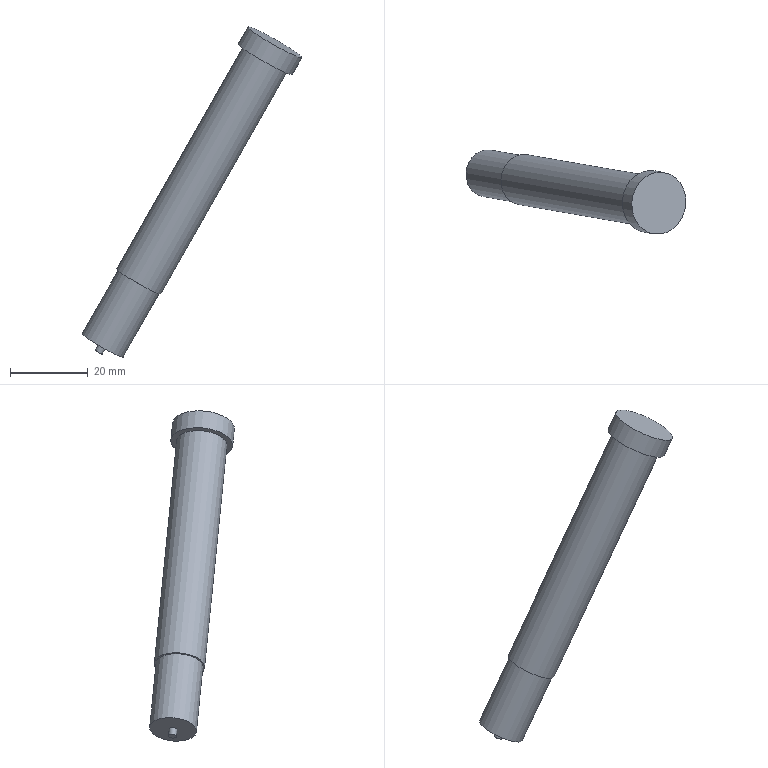Part | NX | features solid 2 | 1 solid | 9 faces | box 56.545 x 21.811 x 84.967 mm | volume 11957 mm3 | plane 5 | cylinder 4 | commonest cylinder face diameters 2 x1 12.1 x1 13 x1 16 x1
STEP:
#1=CARTESIAN_POINT('',(665.66,-168.027,-157.458));
#2=VERTEX_POINT('',#1);
#3=CARTESIAN_POINT('',(661.232,-172.302,-155.369));
#4=DIRECTION('',(0.4924,-0.08682,0.866));
#5=DIRECTION('',(0.6812,0.6577,-0.3214));
#6=AXIS2_PLACEMENT_3D('',#3,#4,#5);
#7=CIRCLE('',#6,6.5);
#8=EDGE_CURVE('',#2,#2,#7,.T.);
#9=ORIENTED_EDGE('',*,*,#8,.T.);
#10=EDGE_LOOP('',(#9));
#11=FACE_BOUND('',#10,.T.);
#12=CARTESIAN_POINT('',(698.159,-173.757,-100.3));
#13=VERTEX_POINT('',#12);
#14=CARTESIAN_POINT('',(693.731,-178.033,-98.211));
#15=DIRECTION('',(0.4924,-0.08682,0.866));
#16=DIRECTION('',(0.6812,0.6577,-0.3214));
#17=AXIS2_PLACEMENT_3D('',#14,#15,#16);
#18=CIRCLE('',#17,6.5);
#19=EDGE_CURVE('',#13,#13,#18,.T.);
#20=ORIENTED_EDGE('',*,*,#19,.F.);
#21=EDGE_LOOP('',(#20));
#22=FACE_BOUND('',#21,.T.);
#23=CARTESIAN_POINT('',(696.193,-178.467,-93.881));
#24=DIRECTION('',(-0.4924,0.08682,-0.866));
#25=DIRECTION('',(-0.6812,-0.6577,0.3214));
#26=AXIS2_PLACEMENT_3D('',#23,#24,#25);
#27=CYLINDRICAL_SURFACE('',#26,6.5);
#28=ADVANCED_FACE('',(#11,#22),#27,.T.);
#29=CARTESIAN_POINT('',(665.354,-168.323,-157.313));
#30=VERTEX_POINT('',#29);
#31=CARTESIAN_POINT('',(661.232,-172.302,-155.369));
#32=DIRECTION('',(0.4924,-0.08682,0.866));
#33=DIRECTION('',(0.6812,0.6577,-0.3214));
#34=AXIS2_PLACEMENT_3D('',#31,#32,#33);
#35=CIRCLE('',#34,6.05);
#36=EDGE_CURVE('',#30,#30,#35,.T.);
#37=ORIENTED_EDGE('',*,*,#36,.T.);
#38=EDGE_LOOP('',(#37));
#39=FACE_BOUND('',#38,.T.);
#40=ORIENTED_EDGE('',*,*,#8,.F.);
#41=EDGE_LOOP('',(#40));
#42=FACE_BOUND('',#41,.T.);
#43=CARTESIAN_POINT('',(661.232,-172.302,-155.369));
#44=DIRECTION('',(0.4924,-0.08682,0.866));
#45=DIRECTION('',(0.6812,0.6577,-0.3214));
#46=AXIS2_PLACEMENT_3D('',#43,#44,#45);
#47=PLANE('',#46);
#48=ADVANCED_FACE('',(#39,#42),#47,.F.);
#49=CARTESIAN_POINT('',(699.181,-172.771,-100.782));
#50=VERTEX_POINT('',#49);
#51=CARTESIAN_POINT('',(693.731,-178.033,-98.211));
#52=DIRECTION('',(0.4924,-0.08682,0.866));
#53=DIRECTION('',(0.6812,0.6577,-0.3214));
#54=AXIS2_PLACEMENT_3D('',#51,#52,#53);
#55=CIRCLE('',#54,8.);
#56=EDGE_CURVE('',#50,#50,#55,.T.);
#57=ORIENTED_EDGE('',*,*,#56,.F.);
#58=EDGE_LOOP('',(#57));
#59=FACE_BOUND('',#58,.T.);
#60=ORIENTED_EDGE('',*,*,#19,.T.);
#61=EDGE_LOOP('',(#60));
#62=FACE_BOUND('',#61,.T.);
#63=CARTESIAN_POINT('',(693.731,-178.033,-98.211));
#64=DIRECTION('',(0.4924,-0.08682,0.866));
#65=DIRECTION('',(0.6812,0.6577,-0.3214));
#66=AXIS2_PLACEMENT_3D('',#63,#64,#65);
#67=PLANE('',#66);
#68=ADVANCED_FACE('',(#59,#62),#67,.F.);
#69=ORIENTED_EDGE('',*,*,#56,.T.);
#70=EDGE_LOOP('',(#69));
#71=FACE_BOUND('',#70,.T.);
#72=CARTESIAN_POINT('',(701.643,-173.205,-96.452));
#73=VERTEX_POINT('',#72);
#74=CARTESIAN_POINT('',(696.193,-178.467,-93.881));
#75=DIRECTION('',(0.4924,-0.08682,0.866));
#76=DIRECTION('',(0.6812,0.6577,-0.3214));
#77=AXIS2_PLACEMENT_3D('',#74,#75,#76);
#78=CIRCLE('',#77,8.);
#79=EDGE_CURVE('',#73,#73,#78,.T.);
#80=ORIENTED_EDGE('',*,*,#79,.F.);
#81=EDGE_LOOP('',(#80));
#82=FACE_BOUND('',#81,.T.);
#83=CARTESIAN_POINT('',(693.731,-178.033,-98.211));
#84=DIRECTION('',(0.4924,-0.08682,0.866));
#85=DIRECTION('',(0.6812,0.6577,-0.3214));
#86=AXIS2_PLACEMENT_3D('',#83,#84,#85);
#87=CYLINDRICAL_SURFACE('',#86,8.);
#88=ADVANCED_FACE('',(#71,#82),#87,.T.);
#89=ORIENTED_EDGE('',*,*,#79,.T.);
#90=EDGE_LOOP('',(#89));
#91=FACE_BOUND('',#90,.T.);
#92=CARTESIAN_POINT('',(696.193,-178.467,-93.881));
#93=DIRECTION('',(0.4924,-0.08682,0.866));
#94=DIRECTION('',(0.6812,0.6577,-0.3214));
#95=AXIS2_PLACEMENT_3D('',#92,#93,#94);
#96=PLANE('',#95);
#97=ADVANCED_FACE('',(#91),#96,.T.);
#98=CARTESIAN_POINT('',(655.998,-166.673,-173.768));
#99=VERTEX_POINT('',#98);
#100=CARTESIAN_POINT('',(651.877,-170.653,-171.823));
#101=DIRECTION('',(0.4924,-0.08682,0.866));
#102=DIRECTION('',(0.6812,0.6577,-0.3214));
#103=AXIS2_PLACEMENT_3D('',#100,#101,#102);
#104=CIRCLE('',#103,6.05);
#105=EDGE_CURVE('',#99,#99,#104,.T.);
#106=ORIENTED_EDGE('',*,*,#105,.T.);
#107=EDGE_LOOP('',(#106));
#108=FACE_BOUND('',#107,.T.);
#109=ORIENTED_EDGE('',*,*,#36,.F.);
#110=EDGE_LOOP('',(#109));
#111=FACE_BOUND('',#110,.T.);
#112=CARTESIAN_POINT('',(651.877,-170.653,-171.823));
#113=DIRECTION('',(0.4924,-0.08682,0.866));
#114=DIRECTION('',(0.6812,0.6577,-0.3214));
#115=AXIS2_PLACEMENT_3D('',#112,#113,#114);
#116=CYLINDRICAL_SURFACE('',#115,6.05);
#117=ADVANCED_FACE('',(#108,#111),#116,.T.);
#118=CARTESIAN_POINT('',(652.558,-169.995,-172.145));
#119=VERTEX_POINT('',#118);
#120=CARTESIAN_POINT('',(651.877,-170.653,-171.823));
#121=DIRECTION('',(0.4924,-0.08682,0.866));
#122=DIRECTION('',(0.6812,0.6577,-0.3214));
#123=AXIS2_PLACEMENT_3D('',#120,#121,#122);
#124=CIRCLE('',#123,1.);
#125=EDGE_CURVE('',#119,#119,#124,.T.);
#126=ORIENTED_EDGE('',*,*,#125,.T.);
#127=EDGE_LOOP('',(#126));
#128=FACE_BOUND('',#127,.T.);
#129=ORIENTED_EDGE('',*,*,#105,.F.);
#130=EDGE_LOOP('',(#129));
#131=FACE_BOUND('',#130,.T.);
#132=CARTESIAN_POINT('',(651.877,-170.653,-171.823));
#133=DIRECTION('',(0.4924,-0.08682,0.866));
#134=DIRECTION('',(0.6812,0.6577,-0.3214));
#135=AXIS2_PLACEMENT_3D('',#132,#133,#134);
#136=PLANE('',#135);
#137=ADVANCED_FACE('',(#128,#131),#136,.F.);
#138=CARTESIAN_POINT('',(651.573,-169.821,-173.877));
#139=VERTEX_POINT('',#138);
#140=CARTESIAN_POINT('',(650.892,-170.479,-173.555));
#141=DIRECTION('',(0.4924,-0.08682,0.866));
#142=DIRECTION('',(0.6812,0.6577,-0.3214));
#143=AXIS2_PLACEMENT_3D('',#140,#141,#142);
#144=CIRCLE('',#143,1.);
#145=EDGE_CURVE('',#139,#139,#144,.T.);
#146=ORIENTED_EDGE('',*,*,#145,.T.);
#147=EDGE_LOOP('',(#146));
#148=FACE_BOUND('',#147,.T.);
#149=ORIENTED_EDGE('',*,*,#125,.F.);
#150=EDGE_LOOP('',(#149));
#151=FACE_BOUND('',#150,.T.);
#152=CARTESIAN_POINT('',(650.892,-170.479,-173.555));
#153=DIRECTION('',(0.4924,-0.08682,0.866));
#154=DIRECTION('',(0.6812,0.6577,-0.3214));
#155=AXIS2_PLACEMENT_3D('',#152,#153,#154);
#156=CYLINDRICAL_SURFACE('',#155,1.);
#157=ADVANCED_FACE('',(#148,#151),#156,.T.);
#158=ORIENTED_EDGE('',*,*,#145,.F.);
#159=EDGE_LOOP('',(#158));
#160=FACE_BOUND('',#159,.T.);
#161=CARTESIAN_POINT('',(650.892,-170.479,-173.555));
#162=DIRECTION('',(0.4924,-0.08682,0.866));
#163=DIRECTION('',(0.6812,0.6577,-0.3214));
#164=AXIS2_PLACEMENT_3D('',#161,#162,#163);
#165=PLANE('',#164);
#166=ADVANCED_FACE('',(#160),#165,.F.);
#167=CLOSED_SHELL('',(#28,#48,#68,#88,#97,#117,#137,#157,#166));
#168=MANIFOLD_SOLID_BREP('',#167);
#169=(LENGTH_UNIT()NAMED_UNIT(*)SI_UNIT(.MILLI.,.METRE.));
#170=UNCERTAINTY_MEASURE_WITH_UNIT(LENGTH_MEASURE(0.00001),#169,'','');
#171=(NAMED_UNIT(*)PLANE_ANGLE_UNIT()SI_UNIT($,.RADIAN.));
#172=(NAMED_UNIT(*)SI_UNIT($,.STERADIAN.)SOLID_ANGLE_UNIT());
#173=(GEOMETRIC_REPRESENTATION_CONTEXT(3)GLOBAL_UNCERTAINTY_ASSIGNED_CONTEXT((#170))GLOBAL_UNIT_ASSIGNED_CONTEXT((#169,#171,#172))REPRESENTATION_CONTEXT('',''));
#174=ADVANCED_BREP_SHAPE_REPRESENTATION('',(#168),#173);